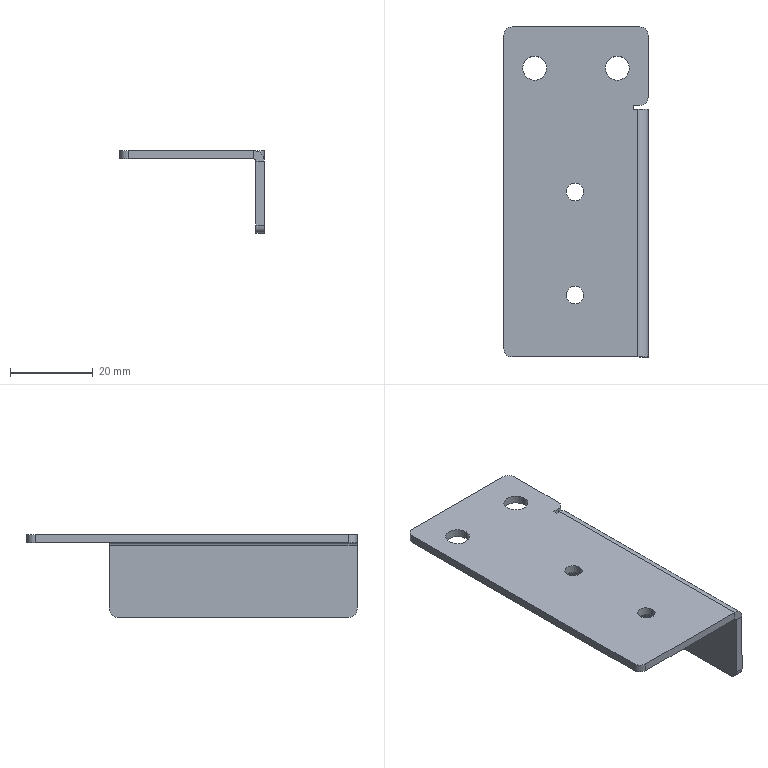Part | SolidWorks | features HoleWzd 2, EdgeFlange 1, Fillet 1, FlatPattern 1, SMBaseFlange 1, SheetMetal 1 | 1 solid | 32 faces | box 35 x 80 x 20 mm | volume 7504 mm3 | cylinder 16 | plane 16 | commonest cylinder face diameters 4 x6 4.2 x4 5.8 x4 1 x1 5 x1
STEP:
#1=CARTESIAN_POINT('',(-2.35,-25.,-2.));
#2=VERTEX_POINT('',#1);
#3=CARTESIAN_POINT('',(1.85,-25.,-2.));
#4=VERTEX_POINT('',#3);
#5=CARTESIAN_POINT('',(-0.25,-25.,-2.));
#6=DIRECTION('',(0.,0.,1.));
#7=DIRECTION('',(1.,0.,0.));
#8=AXIS2_PLACEMENT_3D('',#5,#6,#7);
#9=CIRCLE('',#8,2.1);
#10=EDGE_CURVE('',#2,#4,#9,.T.);
#11=ORIENTED_EDGE('',*,*,#10,.F.);
#12=CARTESIAN_POINT('',(-2.35,-25.,0.));
#13=VERTEX_POINT('',#12);
#14=CARTESIAN_POINT('',(-2.35,-25.,0.));
#15=DIRECTION('',(0.,0.,1.));
#16=VECTOR('',#15,1000.);
#17=LINE('',#14,#16);
#18=EDGE_CURVE('',#2,#13,#17,.T.);
#19=ORIENTED_EDGE('',*,*,#18,.T.);
#20=CARTESIAN_POINT('',(1.85,-25.,0.));
#21=VERTEX_POINT('',#20);
#22=CARTESIAN_POINT('',(-0.25,-25.,0.));
#23=DIRECTION('',(0.,0.,1.));
#24=DIRECTION('',(1.,0.,0.));
#25=AXIS2_PLACEMENT_3D('',#22,#23,#24);
#26=CIRCLE('',#25,2.1);
#27=EDGE_CURVE('',#13,#21,#26,.T.);
#28=ORIENTED_EDGE('',*,*,#27,.T.);
#29=CARTESIAN_POINT('',(1.85,-25.,0.));
#30=DIRECTION('',(0.,0.,1.));
#31=VECTOR('',#30,1000.);
#32=LINE('',#29,#31);
#33=EDGE_CURVE('',#4,#21,#32,.T.);
#34=ORIENTED_EDGE('',*,*,#33,.F.);
#35=EDGE_LOOP('',(#11,#19,#28,#34));
#36=FACE_OUTER_BOUND('',#35,.T.);
#37=CARTESIAN_POINT('',(-0.25,-25.,0.));
#38=DIRECTION('',(0.,0.,1.));
#39=DIRECTION('',(1.,0.,0.));
#40=AXIS2_PLACEMENT_3D('',#37,#38,#39);
#41=CYLINDRICAL_SURFACE('',#40,2.1);
#42=ADVANCED_FACE('',(#36),#41,.F.);
#43=CARTESIAN_POINT('',(-2.35,0.,-2.));
#44=VERTEX_POINT('',#43);
#45=CARTESIAN_POINT('',(1.85,0.,-2.));
#46=VERTEX_POINT('',#45);
#47=CARTESIAN_POINT('',(-0.25,0.,-2.));
#48=DIRECTION('',(0.,0.,1.));
#49=DIRECTION('',(1.,0.,0.));
#50=AXIS2_PLACEMENT_3D('',#47,#48,#49);
#51=CIRCLE('',#50,2.1);
#52=EDGE_CURVE('',#44,#46,#51,.T.);
#53=ORIENTED_EDGE('',*,*,#52,.F.);
#54=CARTESIAN_POINT('',(-2.35,0.,0.));
#55=VERTEX_POINT('',#54);
#56=CARTESIAN_POINT('',(-2.35,0.,0.));
#57=DIRECTION('',(0.,0.,1.));
#58=VECTOR('',#57,1000.);
#59=LINE('',#56,#58);
#60=EDGE_CURVE('',#44,#55,#59,.T.);
#61=ORIENTED_EDGE('',*,*,#60,.T.);
#62=CARTESIAN_POINT('',(1.85,0.,0.));
#63=VERTEX_POINT('',#62);
#64=CARTESIAN_POINT('',(-0.25,0.,0.));
#65=DIRECTION('',(0.,0.,1.));
#66=DIRECTION('',(1.,0.,0.));
#67=AXIS2_PLACEMENT_3D('',#64,#65,#66);
#68=CIRCLE('',#67,2.1);
#69=EDGE_CURVE('',#55,#63,#68,.T.);
#70=ORIENTED_EDGE('',*,*,#69,.T.);
#71=CARTESIAN_POINT('',(1.85,0.,0.));
#72=DIRECTION('',(0.,0.,1.));
#73=VECTOR('',#72,1000.);
#74=LINE('',#71,#73);
#75=EDGE_CURVE('',#46,#63,#74,.T.);
#76=ORIENTED_EDGE('',*,*,#75,.F.);
#77=EDGE_LOOP('',(#53,#61,#70,#76));
#78=FACE_OUTER_BOUND('',#77,.T.);
#79=CARTESIAN_POINT('',(-0.25,0.,0.));
#80=DIRECTION('',(0.,0.,1.));
#81=DIRECTION('',(1.,0.,0.));
#82=AXIS2_PLACEMENT_3D('',#79,#80,#81);
#83=CYLINDRICAL_SURFACE('',#82,2.1);
#84=ADVANCED_FACE('',(#78),#83,.F.);
#85=CARTESIAN_POINT('',(-12.9,30.,-2.));
#86=VERTEX_POINT('',#85);
#87=CARTESIAN_POINT('',(-7.1,30.,-2.));
#88=VERTEX_POINT('',#87);
#89=CARTESIAN_POINT('',(-10.,30.,-2.));
#90=DIRECTION('',(0.,0.,1.));
#91=DIRECTION('',(1.,0.,0.));
#92=AXIS2_PLACEMENT_3D('',#89,#90,#91);
#93=CIRCLE('',#92,2.9);
#94=EDGE_CURVE('',#86,#88,#93,.T.);
#95=ORIENTED_EDGE('',*,*,#94,.F.);
#96=CARTESIAN_POINT('',(-12.9,30.,0.));
#97=VERTEX_POINT('',#96);
#98=CARTESIAN_POINT('',(-12.9,30.,0.));
#99=DIRECTION('',(0.,0.,1.));
#100=VECTOR('',#99,1000.);
#101=LINE('',#98,#100);
#102=EDGE_CURVE('',#86,#97,#101,.T.);
#103=ORIENTED_EDGE('',*,*,#102,.T.);
#104=CARTESIAN_POINT('',(-7.1,30.,0.));
#105=VERTEX_POINT('',#104);
#106=CARTESIAN_POINT('',(-10.,30.,0.));
#107=DIRECTION('',(0.,0.,1.));
#108=DIRECTION('',(1.,0.,0.));
#109=AXIS2_PLACEMENT_3D('',#106,#107,#108);
#110=CIRCLE('',#109,2.9);
#111=EDGE_CURVE('',#97,#105,#110,.T.);
#112=ORIENTED_EDGE('',*,*,#111,.T.);
#113=CARTESIAN_POINT('',(-7.1,30.,0.));
#114=DIRECTION('',(0.,0.,1.));
#115=VECTOR('',#114,1000.);
#116=LINE('',#113,#115);
#117=EDGE_CURVE('',#88,#105,#116,.T.);
#118=ORIENTED_EDGE('',*,*,#117,.F.);
#119=EDGE_LOOP('',(#95,#103,#112,#118));
#120=FACE_OUTER_BOUND('',#119,.T.);
#121=CARTESIAN_POINT('',(-10.,30.,0.));
#122=DIRECTION('',(0.,0.,1.));
#123=DIRECTION('',(1.,0.,0.));
#124=AXIS2_PLACEMENT_3D('',#121,#122,#123);
#125=CYLINDRICAL_SURFACE('',#124,2.9);
#126=ADVANCED_FACE('',(#120),#125,.F.);
#127=CARTESIAN_POINT('',(7.1,30.,-2.));
#128=VERTEX_POINT('',#127);
#129=CARTESIAN_POINT('',(12.9,30.,-2.));
#130=VERTEX_POINT('',#129);
#131=CARTESIAN_POINT('',(10.,30.,-2.));
#132=DIRECTION('',(0.,0.,1.));
#133=DIRECTION('',(1.,0.,0.));
#134=AXIS2_PLACEMENT_3D('',#131,#132,#133);
#135=CIRCLE('',#134,2.9);
#136=EDGE_CURVE('',#128,#130,#135,.T.);
#137=ORIENTED_EDGE('',*,*,#136,.F.);
#138=CARTESIAN_POINT('',(7.1,30.,0.));
#139=VERTEX_POINT('',#138);
#140=CARTESIAN_POINT('',(7.1,30.,0.));
#141=DIRECTION('',(0.,0.,1.));
#142=VECTOR('',#141,1000.);
#143=LINE('',#140,#142);
#144=EDGE_CURVE('',#128,#139,#143,.T.);
#145=ORIENTED_EDGE('',*,*,#144,.T.);
#146=CARTESIAN_POINT('',(12.9,30.,0.));
#147=VERTEX_POINT('',#146);
#148=CARTESIAN_POINT('',(10.,30.,0.));
#149=DIRECTION('',(0.,0.,1.));
#150=DIRECTION('',(1.,0.,0.));
#151=AXIS2_PLACEMENT_3D('',#148,#149,#150);
#152=CIRCLE('',#151,2.9);
#153=EDGE_CURVE('',#139,#147,#152,.T.);
#154=ORIENTED_EDGE('',*,*,#153,.T.);
#155=CARTESIAN_POINT('',(12.9,30.,0.));
#156=DIRECTION('',(0.,0.,1.));
#157=VECTOR('',#156,1000.);
#158=LINE('',#155,#157);
#159=EDGE_CURVE('',#130,#147,#158,.T.);
#160=ORIENTED_EDGE('',*,*,#159,.F.);
#161=EDGE_LOOP('',(#137,#145,#154,#160));
#162=FACE_OUTER_BOUND('',#161,.T.);
#163=CARTESIAN_POINT('',(10.,30.,0.));
#164=DIRECTION('',(0.,0.,1.));
#165=DIRECTION('',(1.,0.,0.));
#166=AXIS2_PLACEMENT_3D('',#163,#164,#165);
#167=CYLINDRICAL_SURFACE('',#166,2.9);
#168=ADVANCED_FACE('',(#162),#167,.F.);
#169=CARTESIAN_POINT('',(17.5,23.,0.));
#170=VERTEX_POINT('',#169);
#171=CARTESIAN_POINT('',(17.5,38.,0.));
#172=VERTEX_POINT('',#171);
#173=CARTESIAN_POINT('',(17.5,-40.,0.));
#174=DIRECTION('',(0.,1.,0.));
#175=VECTOR('',#174,1000.);
#176=LINE('',#173,#175);
#177=EDGE_CURVE('',#170,#172,#176,.T.);
#178=ORIENTED_EDGE('',*,*,#177,.F.);
#179=CARTESIAN_POINT('',(17.5,23.,-2.));
#180=VERTEX_POINT('',#179);
#181=CARTESIAN_POINT('',(17.5,23.,-2.));
#182=DIRECTION('',(0.,0.,-1.));
#183=VECTOR('',#182,1000.);
#184=LINE('',#181,#183);
#185=EDGE_CURVE('',#170,#180,#184,.T.);
#186=ORIENTED_EDGE('',*,*,#185,.T.);
#187=CARTESIAN_POINT('',(17.5,38.,-2.));
#188=VERTEX_POINT('',#187);
#189=CARTESIAN_POINT('',(17.5,-40.,-2.));
#190=DIRECTION('',(0.,1.,0.));
#191=VECTOR('',#190,1000.);
#192=LINE('',#189,#191);
#193=EDGE_CURVE('',#180,#188,#192,.T.);
#194=ORIENTED_EDGE('',*,*,#193,.T.);
#195=CARTESIAN_POINT('',(17.5,38.,-2.));
#196=DIRECTION('',(0.,0.,1.));
#197=VECTOR('',#196,1000.);
#198=LINE('',#195,#197);
#199=EDGE_CURVE('',#188,#172,#198,.T.);
#200=ORIENTED_EDGE('',*,*,#199,.T.);
#201=EDGE_LOOP('',(#178,#186,#194,#200));
#202=FACE_OUTER_BOUND('',#201,.T.);
#203=CARTESIAN_POINT('',(17.5,-40.,-2.));
#204=DIRECTION('',(1.,0.,0.));
#205=DIRECTION('',(0.,0.,-1.));
#206=AXIS2_PLACEMENT_3D('',#203,#204,#205);
#207=PLANE('',#206);
#208=ADVANCED_FACE('',(#202),#207,.T.);
#209=CARTESIAN_POINT('',(-15.5,-40.,0.));
#210=VERTEX_POINT('',#209);
#211=CARTESIAN_POINT('',(15.,-40.,0.));
#212=VERTEX_POINT('',#211);
#213=CARTESIAN_POINT('',(17.5,-40.,0.));
#214=DIRECTION('',(1.,0.,0.));
#215=VECTOR('',#214,1000.);
#216=LINE('',#213,#215);
#217=EDGE_CURVE('',#210,#212,#216,.T.);
#218=ORIENTED_EDGE('',*,*,#217,.F.);
#219=CARTESIAN_POINT('',(-15.5,-40.,-2.));
#220=VERTEX_POINT('',#219);
#221=CARTESIAN_POINT('',(-15.5,-40.,-2.));
#222=DIRECTION('',(0.,0.,-1.));
#223=VECTOR('',#222,1000.);
#224=LINE('',#221,#223);
#225=EDGE_CURVE('',#210,#220,#224,.T.);
#226=ORIENTED_EDGE('',*,*,#225,.T.);
#227=CARTESIAN_POINT('',(15.,-40.,-2.));
#228=VERTEX_POINT('',#227);
#229=CARTESIAN_POINT('',(17.5,-40.,-2.));
#230=DIRECTION('',(1.,0.,0.));
#231=VECTOR('',#230,1000.);
#232=LINE('',#229,#231);
#233=EDGE_CURVE('',#220,#228,#232,.T.);
#234=ORIENTED_EDGE('',*,*,#233,.T.);
#235=CARTESIAN_POINT('',(15.,-40.,-2.));
#236=DIRECTION('',(0.,0.,1.));
#237=VECTOR('',#236,1000.);
#238=LINE('',#235,#237);
#239=EDGE_CURVE('',#228,#212,#238,.T.);
#240=ORIENTED_EDGE('',*,*,#239,.T.);
#241=EDGE_LOOP('',(#218,#226,#234,#240));
#242=FACE_OUTER_BOUND('',#241,.T.);
#243=CARTESIAN_POINT('',(17.5,-40.,-2.));
#244=DIRECTION('',(0.,-1.,0.));
#245=DIRECTION('',(0.,0.,-1.));
#246=AXIS2_PLACEMENT_3D('',#243,#244,#245);
#247=PLANE('',#246);
#248=ADVANCED_FACE('',(#242),#247,.T.);
#249=CARTESIAN_POINT('',(-0.25,-25.,-2.));
#250=DIRECTION('',(0.,0.,1.));
#251=DIRECTION('',(1.,0.,0.));
#252=AXIS2_PLACEMENT_3D('',#249,#250,#251);
#253=CIRCLE('',#252,2.1);
#254=EDGE_CURVE('',#4,#2,#253,.T.);
#255=ORIENTED_EDGE('',*,*,#254,.T.);
#256=ORIENTED_EDGE('',*,*,#10,.T.);
#257=EDGE_LOOP('',(#255,#256));
#258=FACE_BOUND('',#257,.T.);
#259=CARTESIAN_POINT('',(-0.25,0.,-2.));
#260=DIRECTION('',(0.,0.,1.));
#261=DIRECTION('',(1.,0.,0.));
#262=AXIS2_PLACEMENT_3D('',#259,#260,#261);
#263=CIRCLE('',#262,2.1);
#264=EDGE_CURVE('',#46,#44,#263,.T.);
#265=ORIENTED_EDGE('',*,*,#264,.T.);
#266=ORIENTED_EDGE('',*,*,#52,.T.);
#267=EDGE_LOOP('',(#265,#266));
#268=FACE_BOUND('',#267,.T.);
#269=CARTESIAN_POINT('',(-10.,30.,-2.));
#270=DIRECTION('',(0.,0.,1.));
#271=DIRECTION('',(1.,0.,0.));
#272=AXIS2_PLACEMENT_3D('',#269,#270,#271);
#273=CIRCLE('',#272,2.9);
#274=EDGE_CURVE('',#88,#86,#273,.T.);
#275=ORIENTED_EDGE('',*,*,#274,.T.);
#276=ORIENTED_EDGE('',*,*,#94,.T.);
#277=EDGE_LOOP('',(#275,#276));
#278=FACE_BOUND('',#277,.T.);
#279=CARTESIAN_POINT('',(10.,30.,-2.));
#280=DIRECTION('',(0.,0.,1.));
#281=DIRECTION('',(1.,0.,0.));
#282=AXIS2_PLACEMENT_3D('',#279,#280,#281);
#283=CIRCLE('',#282,2.9);
#284=EDGE_CURVE('',#130,#128,#283,.T.);
#285=ORIENTED_EDGE('',*,*,#284,.T.);
#286=ORIENTED_EDGE('',*,*,#136,.T.);
#287=EDGE_LOOP('',(#285,#286));
#288=FACE_BOUND('',#287,.T.);
#289=ORIENTED_EDGE('',*,*,#233,.F.);
#290=CARTESIAN_POINT('',(-17.5,-38.,-2.));
#291=VERTEX_POINT('',#290);
#292=CARTESIAN_POINT('',(-15.5,-38.,-2.));
#293=DIRECTION('',(0.,0.,-1.));
#294=DIRECTION('',(1.,0.,0.));
#295=AXIS2_PLACEMENT_3D('',#292,#293,#294);
#296=CIRCLE('',#295,2.);
#297=EDGE_CURVE('',#220,#291,#296,.T.);
#298=ORIENTED_EDGE('',*,*,#297,.T.);
#299=CARTESIAN_POINT('',(-17.5,38.,-2.));
#300=VERTEX_POINT('',#299);
#301=CARTESIAN_POINT('',(-17.5,-40.,-2.));
#302=DIRECTION('',(0.,-1.,0.));
#303=VECTOR('',#302,1000.);
#304=LINE('',#301,#303);
#305=EDGE_CURVE('',#300,#291,#304,.T.);
#306=ORIENTED_EDGE('',*,*,#305,.F.);
#307=CARTESIAN_POINT('',(-15.5,40.,-2.));
#308=VERTEX_POINT('',#307);
#309=CARTESIAN_POINT('',(-15.5,38.,-2.));
#310=DIRECTION('',(0.,0.,-1.));
#311=DIRECTION('',(1.,0.,0.));
#312=AXIS2_PLACEMENT_3D('',#309,#310,#311);
#313=CIRCLE('',#312,2.);
#314=EDGE_CURVE('',#300,#308,#313,.T.);
#315=ORIENTED_EDGE('',*,*,#314,.T.);
#316=CARTESIAN_POINT('',(15.5,40.,-2.));
#317=VERTEX_POINT('',#316);
#318=CARTESIAN_POINT('',(17.5,40.,-2.));
#319=DIRECTION('',(-1.,0.,0.));
#320=VECTOR('',#319,1000.);
#321=LINE('',#318,#320);
#322=EDGE_CURVE('',#317,#308,#321,.T.);
#323=ORIENTED_EDGE('',*,*,#322,.F.);
#324=CARTESIAN_POINT('',(15.5,38.,-2.));
#325=DIRECTION('',(0.,0.,-1.));
#326=DIRECTION('',(1.,0.,0.));
#327=AXIS2_PLACEMENT_3D('',#324,#325,#326);
#328=CIRCLE('',#327,2.);
#329=EDGE_CURVE('',#317,#188,#328,.T.);
#330=ORIENTED_EDGE('',*,*,#329,.T.);
#331=ORIENTED_EDGE('',*,*,#193,.F.);
#332=CARTESIAN_POINT('',(15.5,21.,-2.));
#333=VERTEX_POINT('',#332);
#334=CARTESIAN_POINT('',(15.5,23.,-2.));
#335=DIRECTION('',(0.,0.,-1.));
#336=DIRECTION('',(1.,0.,0.));
#337=AXIS2_PLACEMENT_3D('',#334,#335,#336);
#338=CIRCLE('',#337,2.);
#339=EDGE_CURVE('',#180,#333,#338,.T.);
#340=ORIENTED_EDGE('',*,*,#339,.T.);
#341=CARTESIAN_POINT('',(14.,21.,-2.));
#342=VERTEX_POINT('',#341);
#343=CARTESIAN_POINT('',(14.,21.,-2.));
#344=DIRECTION('',(1.,0.,0.));
#345=VECTOR('',#344,1000.);
#346=LINE('',#343,#345);
#347=EDGE_CURVE('',#342,#333,#346,.T.);
#348=ORIENTED_EDGE('',*,*,#347,.F.);
#349=CARTESIAN_POINT('',(14.,20.,-2.));
#350=VERTEX_POINT('',#349);
#351=CARTESIAN_POINT('',(14.,20.,-2.));
#352=DIRECTION('',(0.,1.,0.));
#353=VECTOR('',#352,1000.);
#354=LINE('',#351,#353);
#355=EDGE_CURVE('',#350,#342,#354,.T.);
#356=ORIENTED_EDGE('',*,*,#355,.F.);
#357=CARTESIAN_POINT('',(15.,20.,-2.));
#358=VERTEX_POINT('',#357);
#359=CARTESIAN_POINT('',(15.,20.,-2.));
#360=DIRECTION('',(-1.,0.,0.));
#361=VECTOR('',#360,1000.);
#362=LINE('',#359,#361);
#363=EDGE_CURVE('',#358,#350,#362,.T.);
#364=ORIENTED_EDGE('',*,*,#363,.F.);
#365=CARTESIAN_POINT('',(15.,-40.,-2.));
#366=DIRECTION('',(0.,1.,0.));
#367=VECTOR('',#366,1000.);
#368=LINE('',#365,#367);
#369=EDGE_CURVE('',#228,#358,#368,.T.);
#370=ORIENTED_EDGE('',*,*,#369,.F.);
#371=EDGE_LOOP('',(#289,#298,#306,#315,#323,#330,#331,#340,#348,#356,#364,#370));
#372=FACE_OUTER_BOUND('',#371,.T.);
#373=CARTESIAN_POINT('',(0.,0.,-2.));
#374=DIRECTION('',(0.,0.,1.));
#375=DIRECTION('',(1.,0.,0.));
#376=AXIS2_PLACEMENT_3D('',#373,#374,#375);
#377=PLANE('',#376);
#378=ADVANCED_FACE('',(#258,#268,#278,#288,#372),#377,.F.);
#379=CARTESIAN_POINT('',(-0.25,-25.,0.));
#380=DIRECTION('',(0.,0.,1.));
#381=DIRECTION('',(1.,0.,0.));
#382=AXIS2_PLACEMENT_3D('',#379,#380,#381);
#383=CIRCLE('',#382,2.1);
#384=EDGE_CURVE('',#21,#13,#383,.T.);
#385=ORIENTED_EDGE('',*,*,#384,.F.);
#386=ORIENTED_EDGE('',*,*,#27,.F.);
#387=EDGE_LOOP('',(#385,#386));
#388=FACE_BOUND('',#387,.T.);
#389=CARTESIAN_POINT('',(-0.25,0.,0.));
#390=DIRECTION('',(0.,0.,1.));
#391=DIRECTION('',(1.,0.,0.));
#392=AXIS2_PLACEMENT_3D('',#389,#390,#391);
#393=CIRCLE('',#392,2.1);
#394=EDGE_CURVE('',#63,#55,#393,.T.);
#395=ORIENTED_EDGE('',*,*,#394,.F.);
#396=ORIENTED_EDGE('',*,*,#69,.F.);
#397=EDGE_LOOP('',(#395,#396));
#398=FACE_BOUND('',#397,.T.);
#399=CARTESIAN_POINT('',(-10.,30.,0.));
#400=DIRECTION('',(0.,0.,1.));
#401=DIRECTION('',(1.,0.,0.));
#402=AXIS2_PLACEMENT_3D('',#399,#400,#401);
#403=CIRCLE('',#402,2.9);
#404=EDGE_CURVE('',#105,#97,#403,.T.);
#405=ORIENTED_EDGE('',*,*,#404,.F.);
#406=ORIENTED_EDGE('',*,*,#111,.F.);
#407=EDGE_LOOP('',(#405,#406));
#408=FACE_BOUND('',#407,.T.);
#409=CARTESIAN_POINT('',(10.,30.,0.));
#410=DIRECTION('',(0.,0.,1.));
#411=DIRECTION('',(1.,0.,0.));
#412=AXIS2_PLACEMENT_3D('',#409,#410,#411);
#413=CIRCLE('',#412,2.9);
#414=EDGE_CURVE('',#147,#139,#413,.T.);
#415=ORIENTED_EDGE('',*,*,#414,.F.);
#416=ORIENTED_EDGE('',*,*,#153,.F.);
#417=EDGE_LOOP('',(#415,#416));
#418=FACE_BOUND('',#417,.T.);
#419=CARTESIAN_POINT('',(-17.5,38.,0.));
#420=VERTEX_POINT('',#419);
#421=CARTESIAN_POINT('',(-17.5,-38.,0.));
#422=VERTEX_POINT('',#421);
#423=CARTESIAN_POINT('',(-17.5,-40.,0.));
#424=DIRECTION('',(0.,-1.,0.));
#425=VECTOR('',#424,1000.);
#426=LINE('',#423,#425);
#427=EDGE_CURVE('',#420,#422,#426,.T.);
#428=ORIENTED_EDGE('',*,*,#427,.T.);
#429=CARTESIAN_POINT('',(-15.5,-38.,0.));
#430=DIRECTION('',(0.,0.,1.));
#431=DIRECTION('',(1.,0.,0.));
#432=AXIS2_PLACEMENT_3D('',#429,#430,#431);
#433=CIRCLE('',#432,2.);
#434=EDGE_CURVE('',#422,#210,#433,.T.);
#435=ORIENTED_EDGE('',*,*,#434,.T.);
#436=ORIENTED_EDGE('',*,*,#217,.T.);
#437=CARTESIAN_POINT('',(15.,20.,0.));
#438=VERTEX_POINT('',#437);
#439=CARTESIAN_POINT('',(15.,-40.,0.));
#440=DIRECTION('',(0.,1.,0.));
#441=VECTOR('',#440,1000.);
#442=LINE('',#439,#441);
#443=EDGE_CURVE('',#212,#438,#442,.T.);
#444=ORIENTED_EDGE('',*,*,#443,.T.);
#445=CARTESIAN_POINT('',(14.,20.,0.));
#446=VERTEX_POINT('',#445);
#447=CARTESIAN_POINT('',(0.,20.,0.));
#448=DIRECTION('',(-1.,0.,0.));
#449=VECTOR('',#448,1000.);
#450=LINE('',#447,#449);
#451=EDGE_CURVE('',#438,#446,#450,.T.);
#452=ORIENTED_EDGE('',*,*,#451,.T.);
#453=CARTESIAN_POINT('',(14.,21.,0.));
#454=VERTEX_POINT('',#453);
#455=CARTESIAN_POINT('',(14.,0.,0.));
#456=DIRECTION('',(0.,1.,0.));
#457=VECTOR('',#456,1000.);
#458=LINE('',#455,#457);
#459=EDGE_CURVE('',#446,#454,#458,.T.);
#460=ORIENTED_EDGE('',*,*,#459,.T.);
#461=CARTESIAN_POINT('',(15.5,21.,0.));
#462=VERTEX_POINT('',#461);
#463=CARTESIAN_POINT('',(0.,21.,0.));
#464=DIRECTION('',(1.,0.,0.));
#465=VECTOR('',#464,1000.);
#466=LINE('',#463,#465);
#467=EDGE_CURVE('',#454,#462,#466,.T.);
#468=ORIENTED_EDGE('',*,*,#467,.T.);
#469=CARTESIAN_POINT('',(15.5,23.,0.));
#470=DIRECTION('',(0.,0.,1.));
#471=DIRECTION('',(1.,0.,0.));
#472=AXIS2_PLACEMENT_3D('',#469,#470,#471);
#473=CIRCLE('',#472,2.);
#474=EDGE_CURVE('',#462,#170,#473,.T.);
#475=ORIENTED_EDGE('',*,*,#474,.T.);
#476=ORIENTED_EDGE('',*,*,#177,.T.);
#477=CARTESIAN_POINT('',(15.5,40.,0.));
#478=VERTEX_POINT('',#477);
#479=CARTESIAN_POINT('',(15.5,38.,0.));
#480=DIRECTION('',(0.,0.,1.));
#481=DIRECTION('',(1.,0.,0.));
#482=AXIS2_PLACEMENT_3D('',#479,#480,#481);
#483=CIRCLE('',#482,2.);
#484=EDGE_CURVE('',#172,#478,#483,.T.);
#485=ORIENTED_EDGE('',*,*,#484,.T.);
#486=CARTESIAN_POINT('',(-15.5,40.,0.));
#487=VERTEX_POINT('',#486);
#488=CARTESIAN_POINT('',(17.5,40.,0.));
#489=DIRECTION('',(-1.,0.,0.));
#490=VECTOR('',#489,1000.);
#491=LINE('',#488,#490);
#492=EDGE_CURVE('',#478,#487,#491,.T.);
#493=ORIENTED_EDGE('',*,*,#492,.T.);
#494=CARTESIAN_POINT('',(-15.5,38.,0.));
#495=DIRECTION('',(0.,0.,1.));
#496=DIRECTION('',(1.,0.,0.));
#497=AXIS2_PLACEMENT_3D('',#494,#495,#496);
#498=CIRCLE('',#497,2.);
#499=EDGE_CURVE('',#487,#420,#498,.T.);
#500=ORIENTED_EDGE('',*,*,#499,.T.);
#501=EDGE_LOOP('',(#428,#435,#436,#444,#452,#460,#468,#475,#476,#485,#493,#500));
#502=FACE_OUTER_BOUND('',#501,.T.);
#503=CARTESIAN_POINT('',(0.,0.,0.));
#504=DIRECTION('',(0.,0.,1.));
#505=DIRECTION('',(1.,0.,0.));
#506=AXIS2_PLACEMENT_3D('',#503,#504,#505);
#507=PLANE('',#506);
#508=ADVANCED_FACE('',(#388,#398,#408,#418,#502),#507,.T.);
#509=ORIENTED_EDGE('',*,*,#305,.T.);
#510=CARTESIAN_POINT('',(-17.5,-38.,-2.));
#511=DIRECTION('',(0.,0.,1.));
#512=VECTOR('',#511,1000.);
#513=LINE('',#510,#512);
#514=EDGE_CURVE('',#291,#422,#513,.T.);
#515=ORIENTED_EDGE('',*,*,#514,.T.);
#516=ORIENTED_EDGE('',*,*,#427,.F.);
#517=CARTESIAN_POINT('',(-17.5,38.,-2.));
#518=DIRECTION('',(0.,0.,-1.));
#519=VECTOR('',#518,1000.);
#520=LINE('',#517,#519);
#521=EDGE_CURVE('',#420,#300,#520,.T.);
#522=ORIENTED_EDGE('',*,*,#521,.T.);
#523=EDGE_LOOP('',(#509,#515,#516,#522));
#524=FACE_OUTER_BOUND('',#523,.T.);
#525=CARTESIAN_POINT('',(-17.5,-40.,-2.));
#526=DIRECTION('',(-1.,0.,0.));
#527=DIRECTION('',(0.,0.,1.));
#528=AXIS2_PLACEMENT_3D('',#525,#526,#527);
#529=PLANE('',#528);
#530=ADVANCED_FACE('',(#524),#529,.T.);
#531=ORIENTED_EDGE('',*,*,#492,.F.);
#532=CARTESIAN_POINT('',(15.5,40.,-2.));
#533=DIRECTION('',(0.,0.,-1.));
#534=VECTOR('',#533,1000.);
#535=LINE('',#532,#534);
#536=EDGE_CURVE('',#478,#317,#535,.T.);
#537=ORIENTED_EDGE('',*,*,#536,.T.);
#538=ORIENTED_EDGE('',*,*,#322,.T.);
#539=CARTESIAN_POINT('',(-15.5,40.,-2.));
#540=DIRECTION('',(0.,0.,1.));
#541=VECTOR('',#540,1000.);
#542=LINE('',#539,#541);
#543=EDGE_CURVE('',#308,#487,#542,.T.);
#544=ORIENTED_EDGE('',*,*,#543,.T.);
#545=EDGE_LOOP('',(#531,#537,#538,#544));
#546=FACE_OUTER_BOUND('',#545,.T.);
#547=CARTESIAN_POINT('',(17.5,40.,-2.));
#548=DIRECTION('',(0.,1.,0.));
#549=DIRECTION('',(0.,0.,1.));
#550=AXIS2_PLACEMENT_3D('',#547,#548,#549);
#551=PLANE('',#550);
#552=ADVANCED_FACE('',(#546),#551,.T.);
#553=ORIENTED_EDGE('',*,*,#451,.F.);
#554=CARTESIAN_POINT('',(15.,20.,-2.));
#555=DIRECTION('',(0.,0.,1.));
#556=VECTOR('',#555,1000.);
#557=LINE('',#554,#556);
#558=EDGE_CURVE('',#358,#438,#557,.T.);
#559=ORIENTED_EDGE('',*,*,#558,.F.);
#560=ORIENTED_EDGE('',*,*,#363,.T.);
#561=CARTESIAN_POINT('',(14.,20.,-2.));
#562=DIRECTION('',(0.,0.,1.));
#563=VECTOR('',#562,1000.);
#564=LINE('',#561,#563);
#565=EDGE_CURVE('',#350,#446,#564,.T.);
#566=ORIENTED_EDGE('',*,*,#565,.T.);
#567=EDGE_LOOP('',(#553,#559,#560,#566));
#568=FACE_OUTER_BOUND('',#567,.T.);
#569=CARTESIAN_POINT('',(15.,20.,-2.));
#570=DIRECTION('',(0.,1.,0.));
#571=DIRECTION('',(0.,0.,1.));
#572=AXIS2_PLACEMENT_3D('',#569,#570,#571);
#573=PLANE('',#572);
#574=ADVANCED_FACE('',(#568),#573,.T.);
#575=ORIENTED_EDGE('',*,*,#459,.F.);
#576=ORIENTED_EDGE('',*,*,#565,.F.);
#577=ORIENTED_EDGE('',*,*,#355,.T.);
#578=CARTESIAN_POINT('',(14.,21.,-2.));
#579=DIRECTION('',(0.,0.,1.));
#580=VECTOR('',#579,1000.);
#581=LINE('',#578,#580);
#582=EDGE_CURVE('',#342,#454,#581,.T.);
#583=ORIENTED_EDGE('',*,*,#582,.T.);
#584=EDGE_LOOP('',(#575,#576,#577,#583));
#585=FACE_OUTER_BOUND('',#584,.T.);
#586=CARTESIAN_POINT('',(14.,20.,-2.));
#587=DIRECTION('',(1.,0.,0.));
#588=DIRECTION('',(0.,0.,-1.));
#589=AXIS2_PLACEMENT_3D('',#586,#587,#588);
#590=PLANE('',#589);
#591=ADVANCED_FACE('',(#585),#590,.T.);
#592=ORIENTED_EDGE('',*,*,#347,.T.);
#593=CARTESIAN_POINT('',(15.5,21.,-2.));
#594=DIRECTION('',(0.,0.,1.));
#595=VECTOR('',#594,1000.);
#596=LINE('',#593,#595);
#597=EDGE_CURVE('',#333,#462,#596,.T.);
#598=ORIENTED_EDGE('',*,*,#597,.T.);
#599=ORIENTED_EDGE('',*,*,#467,.F.);
#600=ORIENTED_EDGE('',*,*,#582,.F.);
#601=EDGE_LOOP('',(#592,#598,#599,#600));
#602=FACE_OUTER_BOUND('',#601,.T.);
#603=CARTESIAN_POINT('',(14.,21.,-2.));
#604=DIRECTION('',(0.,-1.,0.));
#605=DIRECTION('',(0.,0.,-1.));
#606=AXIS2_PLACEMENT_3D('',#603,#604,#605);
#607=PLANE('',#606);
#608=ADVANCED_FACE('',(#602),#607,.T.);
#609=CARTESIAN_POINT('',(15.5,20.,-2.5));
#610=VERTEX_POINT('',#609);
#611=CARTESIAN_POINT('',(17.5,20.,-2.5));
#612=VERTEX_POINT('',#611);
#613=CARTESIAN_POINT('',(17.5,20.,-2.5));
#614=DIRECTION('',(1.,0.,0.));
#615=VECTOR('',#614,1000.);
#616=LINE('',#613,#615);
#617=EDGE_CURVE('',#610,#612,#616,.T.);
#618=ORIENTED_EDGE('',*,*,#617,.F.);
#619=CARTESIAN_POINT('',(15.,20.,-2.5));
#620=DIRECTION('',(0.,1.,0.));
#621=DIRECTION('',(0.,0.,-1.));
#622=AXIS2_PLACEMENT_3D('',#619,#620,#621);
#623=CIRCLE('',#622,0.5);
#624=EDGE_CURVE('',#358,#610,#623,.T.);
#625=ORIENTED_EDGE('',*,*,#624,.F.);
#626=ORIENTED_EDGE('',*,*,#558,.T.);
#627=CARTESIAN_POINT('',(15.,20.,-2.5));
#628=DIRECTION('',(0.,1.,0.));
#629=DIRECTION('',(0.,0.,-1.));
#630=AXIS2_PLACEMENT_3D('',#627,#628,#629);
#631=CIRCLE('',#630,2.5);
#632=EDGE_CURVE('',#438,#612,#631,.T.);
#633=ORIENTED_EDGE('',*,*,#632,.T.);
#634=EDGE_LOOP('',(#618,#625,#626,#633));
#635=FACE_OUTER_BOUND('',#634,.T.);
#636=CARTESIAN_POINT('',(15.,20.,-2.5));
#637=DIRECTION('',(0.,1.,0.));
#638=DIRECTION('',(0.,0.,1.));
#639=AXIS2_PLACEMENT_3D('',#636,#637,#638);
#640=PLANE('',#639);
#641=ADVANCED_FACE('',(#635),#640,.T.);
#642=CARTESIAN_POINT('',(15.5,-40.,-2.5));
#643=VERTEX_POINT('',#642);
#644=CARTESIAN_POINT('',(15.,-40.,-2.5));
#645=DIRECTION('',(0.,-1.,0.));
#646=DIRECTION('',(0.,0.,-1.));
#647=AXIS2_PLACEMENT_3D('',#644,#645,#646);
#648=CIRCLE('',#647,0.5);
#649=EDGE_CURVE('',#643,#228,#648,.T.);
#650=ORIENTED_EDGE('',*,*,#649,.F.);
#651=CARTESIAN_POINT('',(17.5,-40.,-2.5));
#652=VERTEX_POINT('',#651);
#653=CARTESIAN_POINT('',(15.5,-40.,-2.5));
#654=DIRECTION('',(1.,0.,0.));
#655=VECTOR('',#654,1000.);
#656=LINE('',#653,#655);
#657=EDGE_CURVE('',#643,#652,#656,.T.);
#658=ORIENTED_EDGE('',*,*,#657,.T.);
#659=CARTESIAN_POINT('',(15.,-40.,-2.5));
#660=DIRECTION('',(0.,-1.,0.));
#661=DIRECTION('',(0.,0.,-1.));
#662=AXIS2_PLACEMENT_3D('',#659,#660,#661);
#663=CIRCLE('',#662,2.5);
#664=EDGE_CURVE('',#652,#212,#663,.T.);
#665=ORIENTED_EDGE('',*,*,#664,.T.);
#666=ORIENTED_EDGE('',*,*,#239,.F.);
#667=EDGE_LOOP('',(#650,#658,#665,#666));
#668=FACE_OUTER_BOUND('',#667,.T.);
#669=CARTESIAN_POINT('',(15.,-40.,-2.5));
#670=DIRECTION('',(0.,1.,0.));
#671=DIRECTION('',(0.,0.,1.));
#672=AXIS2_PLACEMENT_3D('',#669,#670,#671);
#673=PLANE('',#672);
#674=ADVANCED_FACE('',(#668),#673,.F.);
#675=ORIENTED_EDGE('',*,*,#443,.F.);
#676=ORIENTED_EDGE('',*,*,#664,.F.);
#677=CARTESIAN_POINT('',(17.5,0.,-2.5));
#678=DIRECTION('',(0.,-1.,0.));
#679=VECTOR('',#678,1000.);
#680=LINE('',#677,#679);
#681=EDGE_CURVE('',#612,#652,#680,.T.);
#682=ORIENTED_EDGE('',*,*,#681,.F.);
#683=ORIENTED_EDGE('',*,*,#632,.F.);
#684=EDGE_LOOP('',(#675,#676,#682,#683));
#685=FACE_OUTER_BOUND('',#684,.T.);
#686=CARTESIAN_POINT('',(15.,-40.,-2.5));
#687=DIRECTION('',(0.,-1.,0.));
#688=DIRECTION('',(1.,0.,0.));
#689=AXIS2_PLACEMENT_3D('',#686,#687,#688);
#690=CYLINDRICAL_SURFACE('',#689,2.5);
#691=ADVANCED_FACE('',(#685),#690,.T.);
#692=ORIENTED_EDGE('',*,*,#369,.T.);
#693=ORIENTED_EDGE('',*,*,#624,.T.);
#694=CARTESIAN_POINT('',(15.5,20.,-2.5));
#695=DIRECTION('',(0.,-1.,0.));
#696=VECTOR('',#695,1000.);
#697=LINE('',#694,#696);
#698=EDGE_CURVE('',#610,#643,#697,.T.);
#699=ORIENTED_EDGE('',*,*,#698,.T.);
#700=ORIENTED_EDGE('',*,*,#649,.T.);
#701=EDGE_LOOP('',(#692,#693,#699,#700));
#702=FACE_OUTER_BOUND('',#701,.T.);
#703=CARTESIAN_POINT('',(15.,-40.,-2.5));
#704=DIRECTION('',(0.,-1.,0.));
#705=DIRECTION('',(1.,0.,0.));
#706=AXIS2_PLACEMENT_3D('',#703,#704,#705);
#707=CYLINDRICAL_SURFACE('',#706,0.5);
#708=ADVANCED_FACE('',(#702),#707,.F.);
#709=CARTESIAN_POINT('',(15.5,-40.,-18.));
#710=VERTEX_POINT('',#709);
#711=CARTESIAN_POINT('',(15.5,-40.,0.));
#712=DIRECTION('',(0.,0.,1.));
#713=VECTOR('',#712,1000.);
#714=LINE('',#711,#713);
#715=EDGE_CURVE('',#710,#643,#714,.T.);
#716=ORIENTED_EDGE('',*,*,#715,.F.);
#717=CARTESIAN_POINT('',(17.5,-40.,-18.));
#718=VERTEX_POINT('',#717);
#719=CARTESIAN_POINT('',(17.5,-40.,-18.));
#720=DIRECTION('',(1.,0.,0.));
#721=VECTOR('',#720,1000.);
#722=LINE('',#719,#721);
#723=EDGE_CURVE('',#710,#718,#722,.T.);
#724=ORIENTED_EDGE('',*,*,#723,.T.);
#725=CARTESIAN_POINT('',(17.5,-40.,-2.));
#726=DIRECTION('',(0.,0.,1.));
#727=VECTOR('',#726,1000.);
#728=LINE('',#725,#727);
#729=EDGE_CURVE('',#718,#652,#728,.T.);
#730=ORIENTED_EDGE('',*,*,#729,.T.);
#731=ORIENTED_EDGE('',*,*,#657,.F.);
#732=EDGE_LOOP('',(#716,#724,#730,#731));
#733=FACE_OUTER_BOUND('',#732,.T.);
#734=CARTESIAN_POINT('',(17.5,-40.,-2.));
#735=DIRECTION('',(0.,-1.,0.));
#736=DIRECTION('',(0.,0.,-1.));
#737=AXIS2_PLACEMENT_3D('',#734,#735,#736);
#738=PLANE('',#737);
#739=ADVANCED_FACE('',(#733),#738,.T.);
#740=CARTESIAN_POINT('',(17.5,20.,-18.));
#741=VERTEX_POINT('',#740);
#742=CARTESIAN_POINT('',(17.5,20.,-20.));
#743=DIRECTION('',(0.,0.,-1.));
#744=VECTOR('',#743,1000.);
#745=LINE('',#742,#744);
#746=EDGE_CURVE('',#612,#741,#745,.T.);
#747=ORIENTED_EDGE('',*,*,#746,.T.);
#748=CARTESIAN_POINT('',(15.5,20.,-18.));
#749=VERTEX_POINT('',#748);
#750=CARTESIAN_POINT('',(17.5,20.,-18.));
#751=DIRECTION('',(-1.,0.,0.));
#752=VECTOR('',#751,1000.);
#753=LINE('',#750,#752);
#754=EDGE_CURVE('',#741,#749,#753,.T.);
#755=ORIENTED_EDGE('',*,*,#754,.T.);
#756=CARTESIAN_POINT('',(15.5,20.,0.));
#757=DIRECTION('',(0.,0.,-1.));
#758=VECTOR('',#757,1000.);
#759=LINE('',#756,#758);
#760=EDGE_CURVE('',#610,#749,#759,.T.);
#761=ORIENTED_EDGE('',*,*,#760,.F.);
#762=ORIENTED_EDGE('',*,*,#617,.T.);
#763=EDGE_LOOP('',(#747,#755,#761,#762));
#764=FACE_OUTER_BOUND('',#763,.T.);
#765=CARTESIAN_POINT('',(17.5,20.,-20.));
#766=DIRECTION('',(0.,1.,0.));
#767=DIRECTION('',(0.,0.,1.));
#768=AXIS2_PLACEMENT_3D('',#765,#766,#767);
#769=PLANE('',#768);
#770=ADVANCED_FACE('',(#764),#769,.T.);
#771=ORIENTED_EDGE('',*,*,#729,.F.);
#772=CARTESIAN_POINT('',(17.5,-38.,-20.));
#773=VERTEX_POINT('',#772);
#774=CARTESIAN_POINT('',(17.5,-38.,-18.));
#775=DIRECTION('',(1.,0.,0.));
#776=DIRECTION('',(0.,0.,-1.));
#777=AXIS2_PLACEMENT_3D('',#774,#775,#776);
#778=CIRCLE('',#777,2.);
#779=EDGE_CURVE('',#718,#773,#778,.T.);
#780=ORIENTED_EDGE('',*,*,#779,.T.);
#781=CARTESIAN_POINT('',(17.5,18.,-20.));
#782=VERTEX_POINT('',#781);
#783=CARTESIAN_POINT('',(17.5,-40.,-20.));
#784=DIRECTION('',(0.,-1.,0.));
#785=VECTOR('',#784,1000.);
#786=LINE('',#783,#785);
#787=EDGE_CURVE('',#782,#773,#786,.T.);
#788=ORIENTED_EDGE('',*,*,#787,.F.);
#789=CARTESIAN_POINT('',(17.5,18.,-18.));
#790=DIRECTION('',(1.,0.,0.));
#791=DIRECTION('',(0.,0.,-1.));
#792=AXIS2_PLACEMENT_3D('',#789,#790,#791);
#793=CIRCLE('',#792,2.);
#794=EDGE_CURVE('',#782,#741,#793,.T.);
#795=ORIENTED_EDGE('',*,*,#794,.T.);
#796=ORIENTED_EDGE('',*,*,#746,.F.);
#797=ORIENTED_EDGE('',*,*,#681,.T.);
#798=EDGE_LOOP('',(#771,#780,#788,#795,#796,#797));
#799=FACE_OUTER_BOUND('',#798,.T.);
#800=CARTESIAN_POINT('',(17.5,0.,0.));
#801=DIRECTION('',(1.,0.,0.));
#802=DIRECTION('',(0.,0.,-1.));
#803=AXIS2_PLACEMENT_3D('',#800,#801,#802);
#804=PLANE('',#803);
#805=ADVANCED_FACE('',(#799),#804,.T.);
#806=CARTESIAN_POINT('',(15.5,18.,-20.));
#807=VERTEX_POINT('',#806);
#808=CARTESIAN_POINT('',(15.5,-38.,-20.));
#809=VERTEX_POINT('',#808);
#810=CARTESIAN_POINT('',(15.5,0.,-20.));
#811=DIRECTION('',(0.,-1.,0.));
#812=VECTOR('',#811,1000.);
#813=LINE('',#810,#812);
#814=EDGE_CURVE('',#807,#809,#813,.T.);
#815=ORIENTED_EDGE('',*,*,#814,.T.);
#816=CARTESIAN_POINT('',(15.5,-38.,-18.));
#817=DIRECTION('',(-1.,0.,0.));
#818=DIRECTION('',(0.,0.,-1.));
#819=AXIS2_PLACEMENT_3D('',#816,#817,#818);
#820=CIRCLE('',#819,2.);
#821=EDGE_CURVE('',#809,#710,#820,.T.);
#822=ORIENTED_EDGE('',*,*,#821,.T.);
#823=ORIENTED_EDGE('',*,*,#715,.T.);
#824=ORIENTED_EDGE('',*,*,#698,.F.);
#825=ORIENTED_EDGE('',*,*,#760,.T.);
#826=CARTESIAN_POINT('',(15.5,18.,-18.));
#827=DIRECTION('',(-1.,0.,0.));
#828=DIRECTION('',(0.,0.,-1.));
#829=AXIS2_PLACEMENT_3D('',#826,#827,#828);
#830=CIRCLE('',#829,2.);
#831=EDGE_CURVE('',#749,#807,#830,.T.);
#832=ORIENTED_EDGE('',*,*,#831,.T.);
#833=EDGE_LOOP('',(#815,#822,#823,#824,#825,#832));
#834=FACE_OUTER_BOUND('',#833,.T.);
#835=CARTESIAN_POINT('',(15.5,0.,0.));
#836=DIRECTION('',(1.,0.,0.));
#837=DIRECTION('',(0.,0.,-1.));
#838=AXIS2_PLACEMENT_3D('',#835,#836,#837);
#839=PLANE('',#838);
#840=ADVANCED_FACE('',(#834),#839,.F.);
#841=ORIENTED_EDGE('',*,*,#787,.T.);
#842=CARTESIAN_POINT('',(17.5,-38.,-20.));
#843=DIRECTION('',(-1.,0.,0.));
#844=VECTOR('',#843,1000.);
#845=LINE('',#842,#844);
#846=EDGE_CURVE('',#773,#809,#845,.T.);
#847=ORIENTED_EDGE('',*,*,#846,.T.);
#848=ORIENTED_EDGE('',*,*,#814,.F.);
#849=CARTESIAN_POINT('',(17.5,18.,-20.));
#850=DIRECTION('',(1.,0.,0.));
#851=VECTOR('',#850,1000.);
#852=LINE('',#849,#851);
#853=EDGE_CURVE('',#807,#782,#852,.T.);
#854=ORIENTED_EDGE('',*,*,#853,.T.);
#855=EDGE_LOOP('',(#841,#847,#848,#854));
#856=FACE_OUTER_BOUND('',#855,.T.);
#857=CARTESIAN_POINT('',(17.5,-40.,-20.));
#858=DIRECTION('',(0.,0.,-1.));
#859=DIRECTION('',(-1.,0.,0.));
#860=AXIS2_PLACEMENT_3D('',#857,#858,#859);
#861=PLANE('',#860);
#862=ADVANCED_FACE('',(#856),#861,.T.);
#863=ORIENTED_EDGE('',*,*,#297,.F.);
#864=ORIENTED_EDGE('',*,*,#225,.F.);
#865=ORIENTED_EDGE('',*,*,#434,.F.);
#866=ORIENTED_EDGE('',*,*,#514,.F.);
#867=EDGE_LOOP('',(#863,#864,#865,#866));
#868=FACE_OUTER_BOUND('',#867,.T.);
#869=CARTESIAN_POINT('',(-15.5,-38.,-2.));
#870=DIRECTION('',(0.,0.,1.));
#871=DIRECTION('',(1.,0.,0.));
#872=AXIS2_PLACEMENT_3D('',#869,#870,#871);
#873=CYLINDRICAL_SURFACE('',#872,2.);
#874=ADVANCED_FACE('',(#868),#873,.T.);
#875=ORIENTED_EDGE('',*,*,#779,.F.);
#876=ORIENTED_EDGE('',*,*,#723,.F.);
#877=ORIENTED_EDGE('',*,*,#821,.F.);
#878=ORIENTED_EDGE('',*,*,#846,.F.);
#879=EDGE_LOOP('',(#875,#876,#877,#878));
#880=FACE_OUTER_BOUND('',#879,.T.);
#881=CARTESIAN_POINT('',(17.5,-38.,-18.));
#882=DIRECTION('',(-1.,0.,0.));
#883=DIRECTION('',(0.,0.,1.));
#884=AXIS2_PLACEMENT_3D('',#881,#882,#883);
#885=CYLINDRICAL_SURFACE('',#884,2.);
#886=ADVANCED_FACE('',(#880),#885,.T.);
#887=ORIENTED_EDGE('',*,*,#794,.F.);
#888=ORIENTED_EDGE('',*,*,#853,.F.);
#889=ORIENTED_EDGE('',*,*,#831,.F.);
#890=ORIENTED_EDGE('',*,*,#754,.F.);
#891=EDGE_LOOP('',(#887,#888,#889,#890));
#892=FACE_OUTER_BOUND('',#891,.T.);
#893=CARTESIAN_POINT('',(17.5,18.,-18.));
#894=DIRECTION('',(-1.,0.,0.));
#895=DIRECTION('',(0.,0.,1.));
#896=AXIS2_PLACEMENT_3D('',#893,#894,#895);
#897=CYLINDRICAL_SURFACE('',#896,2.);
#898=ADVANCED_FACE('',(#892),#897,.T.);
#899=ORIENTED_EDGE('',*,*,#339,.F.);
#900=ORIENTED_EDGE('',*,*,#185,.F.);
#901=ORIENTED_EDGE('',*,*,#474,.F.);
#902=ORIENTED_EDGE('',*,*,#597,.F.);
#903=EDGE_LOOP('',(#899,#900,#901,#902));
#904=FACE_OUTER_BOUND('',#903,.T.);
#905=CARTESIAN_POINT('',(15.5,23.,-2.));
#906=DIRECTION('',(0.,0.,1.));
#907=DIRECTION('',(1.,0.,0.));
#908=AXIS2_PLACEMENT_3D('',#905,#906,#907);
#909=CYLINDRICAL_SURFACE('',#908,2.);
#910=ADVANCED_FACE('',(#904),#909,.T.);
#911=ORIENTED_EDGE('',*,*,#329,.F.);
#912=ORIENTED_EDGE('',*,*,#536,.F.);
#913=ORIENTED_EDGE('',*,*,#484,.F.);
#914=ORIENTED_EDGE('',*,*,#199,.F.);
#915=EDGE_LOOP('',(#911,#912,#913,#914));
#916=FACE_OUTER_BOUND('',#915,.T.);
#917=CARTESIAN_POINT('',(15.5,38.,-2.));
#918=DIRECTION('',(0.,0.,1.));
#919=DIRECTION('',(1.,0.,0.));
#920=AXIS2_PLACEMENT_3D('',#917,#918,#919);
#921=CYLINDRICAL_SURFACE('',#920,2.);
#922=ADVANCED_FACE('',(#916),#921,.T.);
#923=ORIENTED_EDGE('',*,*,#314,.F.);
#924=ORIENTED_EDGE('',*,*,#521,.F.);
#925=ORIENTED_EDGE('',*,*,#499,.F.);
#926=ORIENTED_EDGE('',*,*,#543,.F.);
#927=EDGE_LOOP('',(#923,#924,#925,#926));
#928=FACE_OUTER_BOUND('',#927,.T.);
#929=CARTESIAN_POINT('',(-15.5,38.,-2.));
#930=DIRECTION('',(0.,0.,1.));
#931=DIRECTION('',(1.,0.,0.));
#932=AXIS2_PLACEMENT_3D('',#929,#930,#931);
#933=CYLINDRICAL_SURFACE('',#932,2.);
#934=ADVANCED_FACE('',(#928),#933,.T.);
#935=ORIENTED_EDGE('',*,*,#144,.F.);
#936=ORIENTED_EDGE('',*,*,#284,.F.);
#937=ORIENTED_EDGE('',*,*,#159,.T.);
#938=ORIENTED_EDGE('',*,*,#414,.T.);
#939=EDGE_LOOP('',(#935,#936,#937,#938));
#940=FACE_OUTER_BOUND('',#939,.T.);
#941=CARTESIAN_POINT('',(10.,30.,0.));
#942=DIRECTION('',(0.,0.,1.));
#943=DIRECTION('',(1.,0.,0.));
#944=AXIS2_PLACEMENT_3D('',#941,#942,#943);
#945=CYLINDRICAL_SURFACE('',#944,2.9);
#946=ADVANCED_FACE('',(#940),#945,.F.);
#947=ORIENTED_EDGE('',*,*,#102,.F.);
#948=ORIENTED_EDGE('',*,*,#274,.F.);
#949=ORIENTED_EDGE('',*,*,#117,.T.);
#950=ORIENTED_EDGE('',*,*,#404,.T.);
#951=EDGE_LOOP('',(#947,#948,#949,#950));
#952=FACE_OUTER_BOUND('',#951,.T.);
#953=CARTESIAN_POINT('',(-10.,30.,0.));
#954=DIRECTION('',(0.,0.,1.));
#955=DIRECTION('',(1.,0.,0.));
#956=AXIS2_PLACEMENT_3D('',#953,#954,#955);
#957=CYLINDRICAL_SURFACE('',#956,2.9);
#958=ADVANCED_FACE('',(#952),#957,.F.);
#959=ORIENTED_EDGE('',*,*,#60,.F.);
#960=ORIENTED_EDGE('',*,*,#264,.F.);
#961=ORIENTED_EDGE('',*,*,#75,.T.);
#962=ORIENTED_EDGE('',*,*,#394,.T.);
#963=EDGE_LOOP('',(#959,#960,#961,#962));
#964=FACE_OUTER_BOUND('',#963,.T.);
#965=CARTESIAN_POINT('',(-0.25,0.,0.));
#966=DIRECTION('',(0.,0.,1.));
#967=DIRECTION('',(1.,0.,0.));
#968=AXIS2_PLACEMENT_3D('',#965,#966,#967);
#969=CYLINDRICAL_SURFACE('',#968,2.1);
#970=ADVANCED_FACE('',(#964),#969,.F.);
#971=ORIENTED_EDGE('',*,*,#18,.F.);
#972=ORIENTED_EDGE('',*,*,#254,.F.);
#973=ORIENTED_EDGE('',*,*,#33,.T.);
#974=ORIENTED_EDGE('',*,*,#384,.T.);
#975=EDGE_LOOP('',(#971,#972,#973,#974));
#976=FACE_OUTER_BOUND('',#975,.T.);
#977=CARTESIAN_POINT('',(-0.25,-25.,0.));
#978=DIRECTION('',(0.,0.,1.));
#979=DIRECTION('',(1.,0.,0.));
#980=AXIS2_PLACEMENT_3D('',#977,#978,#979);
#981=CYLINDRICAL_SURFACE('',#980,2.1);
#982=ADVANCED_FACE('',(#976),#981,.F.);
#983=CLOSED_SHELL('',(#42,#84,#126,#168,#208,#248,#378,#508,#530,#552,#574,#591,#608,#641,#674,#691,#708,#739,#770,#805,#840,#862,#874,#886,#898,#910,#922,#934,#946,#958,#970,#982));
#984=MANIFOLD_SOLID_BREP('',#983);
#985=CARTESIAN_POINT('',(0.,0.,0.));
#986=DIRECTION('',(0.,0.,1.));
#987=DIRECTION('',(1.,0.,0.));
#988=AXIS2_PLACEMENT_3D('',#985,#986,#987);
#989=(LENGTH_UNIT()NAMED_UNIT(*)SI_UNIT(.MILLI.,.METRE.));
#990=UNCERTAINTY_MEASURE_WITH_UNIT(LENGTH_MEASURE(0.00001),#989,'','');
#991=(NAMED_UNIT(*)PLANE_ANGLE_UNIT()SI_UNIT($,.RADIAN.));
#992=(NAMED_UNIT(*)SI_UNIT($,.STERADIAN.)SOLID_ANGLE_UNIT());
#993=(GEOMETRIC_REPRESENTATION_CONTEXT(3)GLOBAL_UNCERTAINTY_ASSIGNED_CONTEXT((#990))GLOBAL_UNIT_ASSIGNED_CONTEXT((#989,#991,#992))REPRESENTATION_CONTEXT('',''));
#994=ADVANCED_BREP_SHAPE_REPRESENTATION('',(#984,#988),#993);